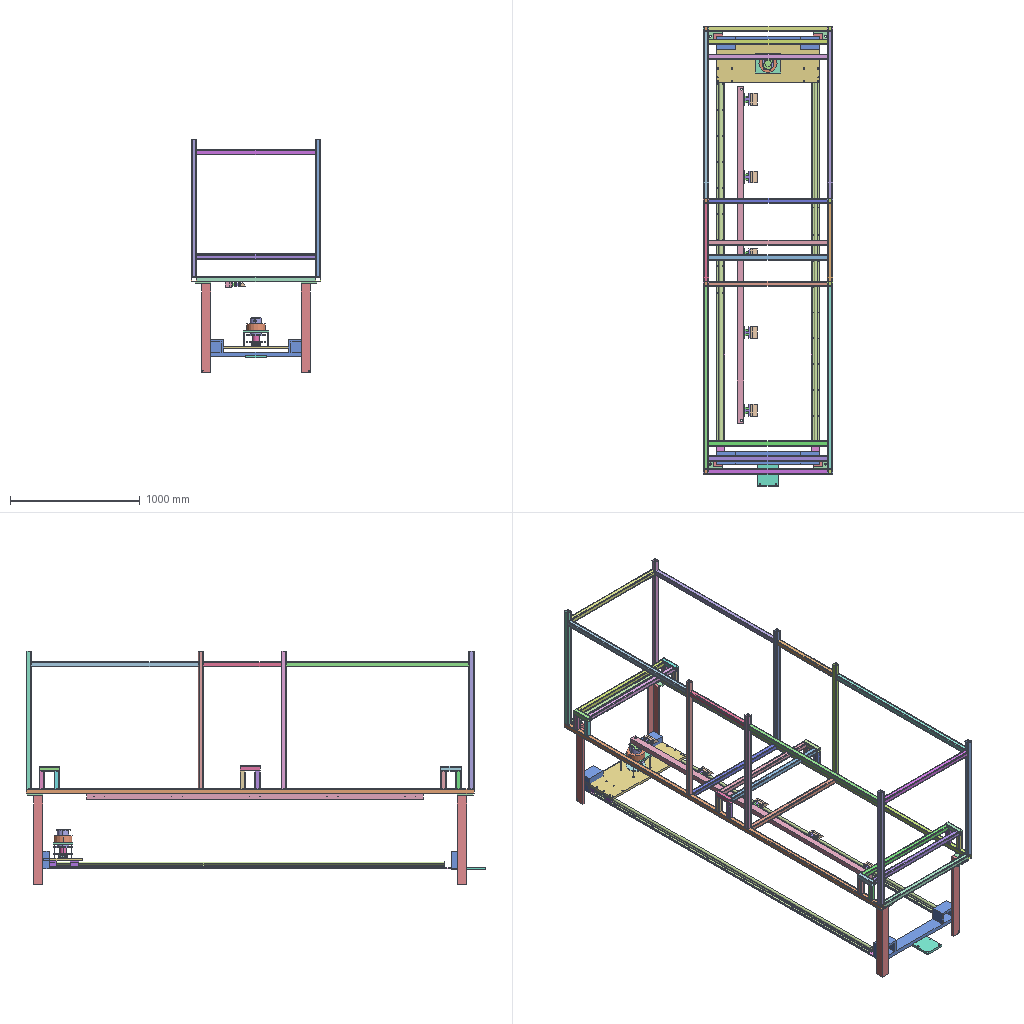Assembly | SolidWorks | 20 different items | 41 placed | box 996 x 3546 x 1800 mm
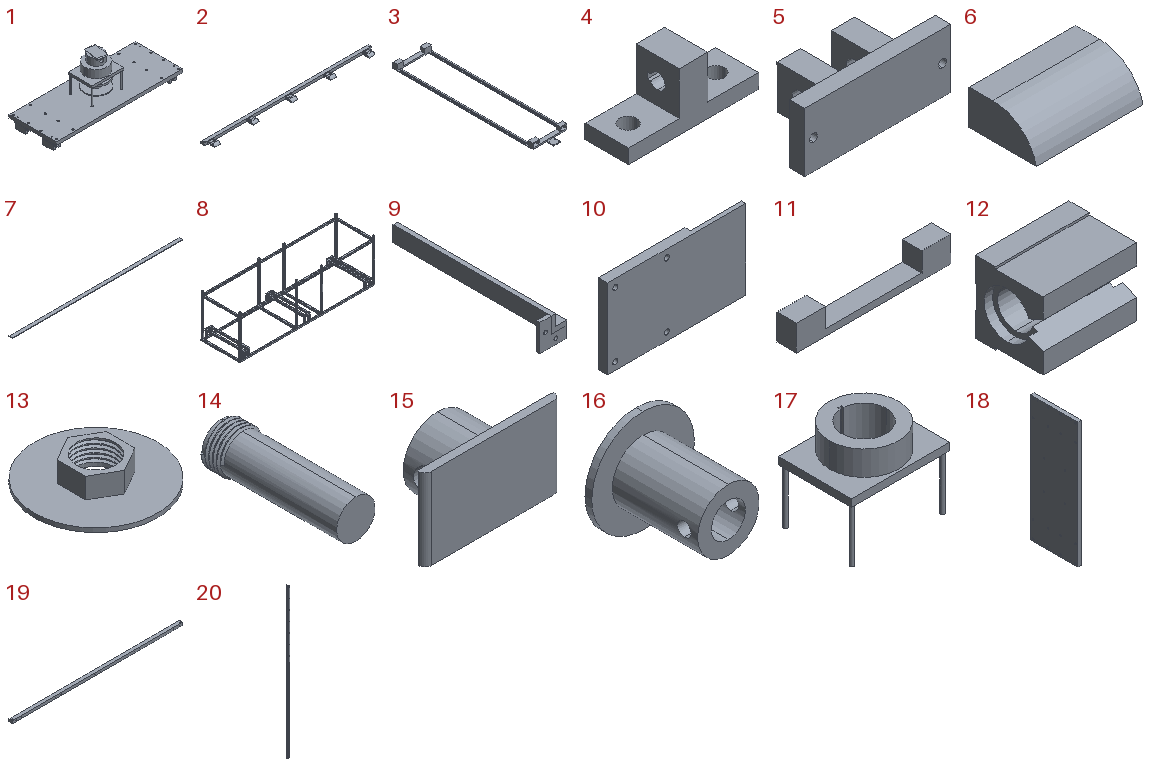Parts list (item | name | quantity | parent item | size | volume | features):
1 | (subassembly) | x1 | - | 800 x 300 x 287.288 mm | 7220529 mm3 | features CompositeCurve 6
2 | (subassembly) | x1 | - | 2596 x 157.44 x 40 mm | 6283674 mm3 | features ReferencePattern 12, CompositeCurve 9, LocalLPattern 1
3 | (subassembly) | x1 | - | 800 x 3468 x 142 mm | 18121167 mm3 | -
4 | - | x5 | in 2 | 91 x 30 x 40 mm | 41147 mm3 | features ICE 3, Extrusion 1
5 | - | x5 | in 2 | 94 x 40 x 38 mm | 57385 mm3 | features ICE 5, Extrusion 1, MirrorPattern 1
6 | - | x5 | in 2 | 91 x 57.44 x 30 mm | 125435 mm3 | features SweepThread 2, Extrusion 1, Fillet 1, ICE 1
7 | - | x2 | in 3 | 3100 x 65 x 8 mm | 1612000 mm3 | features Extrusion 1
8 | - | x1 | - | 3455 x 996 x 1100 mm | 14945108 mm3 | features WeldCornerFeat 8, 3DProfileFeature 1, MirrorSolid 1, WeldMemberFeat 1, WeldmentFeature 1
9 | - | x4 | - | 120 x 700 x 120 mm | 1815903 mm3 | features ICE 2, Extrusion 1
10 | - | x1 | in 3 | 268.5 x 18 x 155 mm | 588460 mm3 | features ICE 2, Extrusion 1
11 | - | x2 | in 3 | 800 x 100 x 134 mm | 4312000 mm3 | features Split 3, Cut 2, Extrusion 1, MirrorPattern 1
12 | - | x4 | in 1 | 65 x 47 x 50 mm | 97950 mm3 | features 3DProfileFeature 2, HoleWzd 2, ICE 2, Extrusion 1
13 | - | x1 | in 1 | 150 x 150 x 30 mm | 107137 mm3 | features ICE 2, Cut 1, Extrusion 1, SweepThread 1
14 | - | x1 | in 1 | 55.413 x 175 x 55.413 mm | 348440 mm3 | features Extrusion 1, SweepThread 1
15 | - | x1 | in 1 | 100 x 41 x 60 mm | 88631 mm3 | features ICE 2, Chamfer 1, Extrusion 1, Fillet 1
16 | - | x1 | in 1 | 150 x 135 x 150 mm | 694147 mm3 | features ICE 2, Extrusion 1
17 | - | x1 | in 1 | 200 x 150 x 175 mm | 822892 mm3 | features ICE 4, Cut 1, Extrusion 1
18 | - | x1 | in 1 | 20 x 300 x 800 mm | 4767476 mm3 | features ICE 3, Extrusion 1
19 | - | x1 | in 2 | 2596 x 50 x 40 mm | 5166098 mm3 | features ICE 2, Extrusion 1
20 | - | x2 | in 3 | 55 x 45.5 x 3000 mm | 2842353 mm3 | features Chamfer 1, Extrusion 1, ICE 1, MoveFace 1
Mates (type | each side: item.copy, entity, surface, feature):
In the top assembly
DistanceDim | 8.1 face plane Structural cold-formed square hollow steel (gb t6728-2002) 40×3(8) | assembly face
Coincident | assembly face | 8.1 face plane Structural cold-formed square hollow steel (gb t6728-2002) 40×3(8)
DistanceDim | assembly face | 8.1 face plane Structural cold-formed square hollow steel (gb t6728-2002) 40×3(8)
Concentric | assembly face | assembly edge | 8 times
Parallel | assembly face | assembly face | 4 times
Coincident | assembly face | assembly face
Concentric | assembly face | 17.1 face cylinder Boss-Extrude3
Concentric | assembly edge | 17.1 face cylinder Boss-Extrude3
DistanceDim | 17.1 face plane Boss-Extrude3 | assembly face
Coincident | 8.1 face plane Structural cold-formed square hollow steel (gb t6728-2002) 40×3(8) | 9.1 face plane Boss-Extrude1
Coincident | 9.1 face plane Boss-Extrude2 | 11.1 face plane Boss-Extrude1 | 2 times
Concentric | assembly edge | 20.1 face cylinder Boss-Extrude1
Concentric | 12.1 face cylinder Extrude1 | 20.1 face cylinder Boss-Extrude1
Concentric | 12.2 face cylinder Extrude1 | 20.2 face cylinder Boss-Extrude1
Coincident | 11.2 face plane Boss-Extrude1 | 9.2 face plane Boss-Extrude2 | 2 times
Coincident | 8.1 face plane Structural cold-formed square hollow steel (gb t6728-2002) 40×3(8) | 9.2 face plane Boss-Extrude1
Coincident | 11.2 face plane Boss-Extrude1 | 9.3 face plane Boss-Extrude2 | 2 times
Coincident | 8.1 face plane Structural cold-formed square hollow steel (gb t6728-2002) 40×3(8) | 9.3 face plane Boss-Extrude1
Coincident | 8.1 face plane Structural cold-formed square hollow steel (gb t6728-2002) 40×3(8) | 9.4 face plane Boss-Extrude1
Coincident | 11.1 face plane Boss-Extrude1 | 9.4 face plane Boss-Extrude2 | 2 times
Coincident | 8.1 face plane Structural cold-formed square hollow steel (gb t6728-2002) 40×3(8) | 19.1 face plane Boss-Extrude1
In subassembly 3
Coincident | 3.1 face | 3.1 face | 3 times
DistanceDim | 20.3 face plane Boss-Extrude1 | 11.3 face plane Boss-Extrude1
Coincident | 11.3 face plane Boss-Extrude1 | 7.1 face plane Boss-Extrude1 | 3 times
DistanceDim | 7.1 face plane Boss-Extrude1 | 20.3 face plane Boss-Extrude1
DistanceDim | 11.3 face plane Boss-Extrude1 | 20.3 face plane Boss-Extrude1
Coincident | 11.3 face plane Boss-Extrude1 | 7.2 face plane Boss-Extrude1 | 3 times
DistanceDim | 20.4 face plane Boss-Extrude1 | 7.2 face plane Boss-Extrude1
DistanceDim | 20.4 face plane Boss-Extrude1 | 11.3 face plane Boss-Extrude1
Coincident | 7.2 face plane Boss-Extrude1 | 20.4 face plane Boss-Extrude1
Coincident | 7.2 face plane Boss-Extrude1 | 3.1 face
Coincident | 7.1 face plane Boss-Extrude1 | 3.1 face
Coincident | 3.1 face | 11.4 face plane Boss-Extrude1 | 3 times
Coincident | 7.1 face plane Boss-Extrude1 | 11.4 face plane Boss-Extrude1 | 2 times
Coincident | 11.3 face plane Boss-Extrude1 | 10.1 face plane Cut-Extrude2
DistanceDim | 10.1 face plane Boss-Extrude1 | 3.1 face
Coincident | 11.4 face plane Boss-Extrude1 | 10.1 face plane Cut-Extrude2
DistanceDim | 10.1 face plane Boss-Extrude1 | 11.4 face plane Boss-Extrude1
Coincident | 7.2 face plane Boss-Extrude1 | 11.4 face plane Boss-Extrude1
In subassembly 1
Concentric | 17.2 face cylinder Boss-Extrude1 | 16.1 face cylinder Boss-Extrude2
Concentric | 16.1 face cylinder Cut-Extrude1 | 15.1 face cylinder Cut-Extrude1
Parallel | 16.1 face plane Boss-Extrude2 | 15.1 face plane Boss-Extrude2
Concentric | 16.1 face cylinder Boss-Extrude1 | 15.1 face cylinder Boss-Extrude1
Concentric | 16.1 face cylinder Boss-Extrude1 | 14.1 face cylinder Boss-Extrude1
Coincident | 15.1 face plane Boss-Extrude1 | 14.1 face plane Boss-Extrude1
Concentric | 14.1 edge | 13.1 edge
Coincident | 14.1 face plane Boss-Extrude1 | 13.1 face plane Boss-Extrude2
DistanceDim | 17.2 face plane Boss-Extrude2 | 16.1 face plane Boss-Extrude1
Concentric | 17.2 edge | 18.1 edge
Concentric | 17.2 face cylinder Boss-Extrude3 | 18.1 edge
Concentric | 17.2 face cylinder Boss-Extrude3 | 18.1 face cylinder Cut-Extrude3
DistanceDim | 18.1 face plane Boss-Extrude1 | 17.2 face plane Boss-Extrude3
Concentric | 18.1 face cylinder Cut-Extrude2 | 12.3 face cylinder M5x0.8 Tapped Hole1
Parallel | 18.1 face plane Boss-Extrude1 | 12.3 face plane Extrude1
Concentric | 18.1 face cylinder Cut-Extrude2 | 12.4 face cylinder M5x0.8 Tapped Hole1
Parallel | 18.1 face plane Boss-Extrude1 | 12.4 face plane Extrude1
Concentric | 18.1 face cylinder Cut-Extrude2 | 12.5 face cylinder M5x0.8 Tapped Hole1
Parallel | 18.1 face plane Boss-Extrude1 | 12.5 face plane Extrude1
Concentric | 18.1 face cylinder Cut-Extrude2 | 12.6 face cylinder M5x0.8 Tapped Hole1
Parallel | 18.1 face plane Boss-Extrude1 | 12.6 face plane Extrude1
In subassembly 2
Concentric | 6.1 edge | 4.1 face cylinder Cut-Extrude2 | 2 times
Coincident | 6.1 face plane Boss-Extrude1 | 4.1 face plane Boss-Extrude1
Coincident | 4.1 face plane Boss-Extrude2 | 5.1 face plane Boss-Extrude2
Concentric | 4.1 edge | 5.1 edge
Concentric | 5.1 face cylinder Mirror1 | 19.2 edge
Concentric | 5.1 edge | 19.2 edge
Parallel | 6.1 face plane Boss-Extrude1 | 19.2 face plane Boss-Extrude1
Coincident | 5.1 face plane Boss-Extrude1 | 19.2 face plane Boss-Extrude1